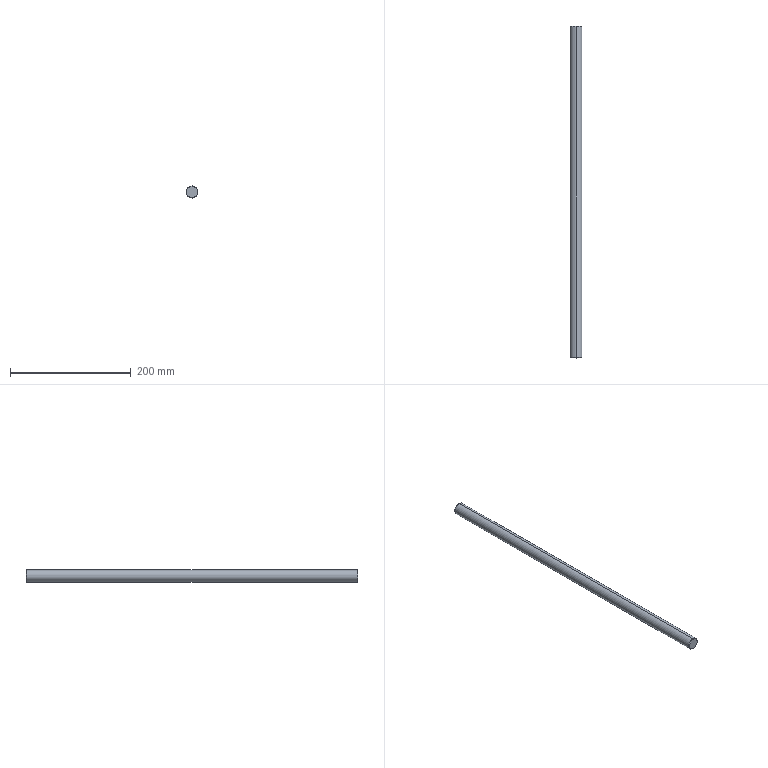Part | STEP file | BCC3 H16_11 | 1 solid | 8 faces | box 20 x 550 x 20 mm | volume 172727 mm3 | cone 4 | cylinder 2 | plane 2 | commonest cylinder face diameters 20 x2
STEP:
#1=CARTESIAN_POINT('',(0.,0.,0.));
#2=DIRECTION('',(0.,0.,1.));
#3=DIRECTION('',(1.,0.,0.));
#4=AXIS2_PLACEMENT_3D('',#1,#2,#3);
#5=CARTESIAN_POINT('',(0.,550.,9.));
#6=VERTEX_POINT('',#5);
#7=CARTESIAN_POINT('',(0.,550.,-9.));
#8=VERTEX_POINT('',#7);
#9=CARTESIAN_POINT('',(0.,550.,0.));
#10=DIRECTION('',(0.,1.,0.));
#11=DIRECTION('',(0.,0.,1.));
#12=AXIS2_PLACEMENT_3D('',#9,#10,#11);
#13=CIRCLE('',#12,9.);
#14=CARTESIAN_POINT('',(0.,550.,0.));
#15=DIRECTION('',(0.,-1.,0.));
#16=DIRECTION('',(0.,0.,-1.));
#17=AXIS2_PLACEMENT_3D('',#14,#15,#16);
#18=CONICAL_SURFACE('',#17,9.,0.7854);
#19=CARTESIAN_POINT('',(3.142,0.));
#20=DIRECTION('',(-1.,0.));
#21=VECTOR('',#20,1.);
#22=LINE('',#19,#21);
#23=(GEOMETRIC_REPRESENTATION_CONTEXT(2)PARAMETRIC_REPRESENTATION_CONTEXT()REPRESENTATION_CONTEXT('',''));
#24=DEFINITIONAL_REPRESENTATION('',(#22),#23);
#25=PCURVE('',#18,#24);
#26=CARTESIAN_POINT('',(0.,550.,0.));
#27=DIRECTION('',(0.,1.,0.));
#28=DIRECTION('',(0.,0.,1.));
#29=AXIS2_PLACEMENT_3D('',#26,#27,#28);
#30=PLANE('',#29);
#31=CARTESIAN_POINT('',(0.,0.));
#32=DIRECTION('',(1.,0.));
#33=AXIS2_PLACEMENT_2D('',#31,#32);
#34=CIRCLE('',#33,9.);
#35=(GEOMETRIC_REPRESENTATION_CONTEXT(2)PARAMETRIC_REPRESENTATION_CONTEXT()REPRESENTATION_CONTEXT('',''));
#36=DEFINITIONAL_REPRESENTATION('',(#34),#35);
#37=PCURVE('',#30,#36);
#38=SURFACE_CURVE('',#13,(#25,#37),.PCURVE_S1.);
#39=EDGE_CURVE('',#6,#8,#38,.T.);
#40=ORIENTED_EDGE('',*,*,#39,.F.);
#41=CARTESIAN_POINT('',(0.,549.,10.));
#42=VERTEX_POINT('',#41);
#43=CARTESIAN_POINT('',(0.,550.,9.));
#44=DIRECTION('',(0.,-0.7071,0.7071));
#45=VECTOR('',#44,1.);
#46=LINE('',#43,#45);
#47=CARTESIAN_POINT('',(3.142,0.));
#48=DIRECTION('',(0.,1.));
#49=VECTOR('',#48,1.);
#50=LINE('',#47,#49);
#51=(GEOMETRIC_REPRESENTATION_CONTEXT(2)PARAMETRIC_REPRESENTATION_CONTEXT()REPRESENTATION_CONTEXT('',''));
#52=DEFINITIONAL_REPRESENTATION('',(#50),#51);
#53=PCURVE('',#18,#52);
#54=CARTESIAN_POINT('',(0.,550.,0.));
#55=DIRECTION('',(0.,-1.,0.));
#56=DIRECTION('',(0.,0.,-1.));
#57=AXIS2_PLACEMENT_3D('',#54,#55,#56);
#58=CONICAL_SURFACE('',#57,9.,0.7854);
#59=CARTESIAN_POINT('',(3.142,0.));
#60=DIRECTION('',(0.,1.));
#61=VECTOR('',#60,1.);
#62=LINE('',#59,#61);
#63=(GEOMETRIC_REPRESENTATION_CONTEXT(2)PARAMETRIC_REPRESENTATION_CONTEXT()REPRESENTATION_CONTEXT('',''));
#64=DEFINITIONAL_REPRESENTATION('',(#62),#63);
#65=PCURVE('',#58,#64);
#66=SURFACE_CURVE('',#46,(#53,#65),.PCURVE_S1.);
#67=EDGE_CURVE('',#6,#42,#66,.T.);
#68=ORIENTED_EDGE('',*,*,#67,.T.);
#69=CARTESIAN_POINT('',(0.,549.,-10.));
#70=VERTEX_POINT('',#69);
#71=CARTESIAN_POINT('',(0.,549.,0.));
#72=DIRECTION('',(0.,-1.,0.));
#73=DIRECTION('',(0.,0.,1.));
#74=AXIS2_PLACEMENT_3D('',#71,#72,#73);
#75=CIRCLE('',#74,10.);
#76=CARTESIAN_POINT('',(-3.142,1.));
#77=DIRECTION('',(1.,0.));
#78=VECTOR('',#77,1.);
#79=LINE('',#76,#78);
#80=(GEOMETRIC_REPRESENTATION_CONTEXT(2)PARAMETRIC_REPRESENTATION_CONTEXT()REPRESENTATION_CONTEXT('',''));
#81=DEFINITIONAL_REPRESENTATION('',(#79),#80);
#82=PCURVE('',#18,#81);
#83=CARTESIAN_POINT('',(0.,550.,0.));
#84=DIRECTION('',(0.,-1.,0.));
#85=DIRECTION('',(0.,0.,-1.));
#86=AXIS2_PLACEMENT_3D('',#83,#84,#85);
#87=CYLINDRICAL_SURFACE('',#86,10.);
#88=CARTESIAN_POINT('',(-3.142,1.));
#89=DIRECTION('',(1.,0.));
#90=VECTOR('',#89,1.);
#91=LINE('',#88,#90);
#92=(GEOMETRIC_REPRESENTATION_CONTEXT(2)PARAMETRIC_REPRESENTATION_CONTEXT()REPRESENTATION_CONTEXT('',''));
#93=DEFINITIONAL_REPRESENTATION('',(#91),#92);
#94=PCURVE('',#87,#93);
#95=SURFACE_CURVE('',#75,(#82,#94),.PCURVE_S1.);
#96=EDGE_CURVE('',#70,#42,#95,.T.);
#97=ORIENTED_EDGE('',*,*,#96,.F.);
#98=CARTESIAN_POINT('',(0.,550.,-9.));
#99=DIRECTION('',(0.,-0.7071,-0.7071));
#100=VECTOR('',#99,1.);
#101=LINE('',#98,#100);
#102=CARTESIAN_POINT('',(0.,0.));
#103=DIRECTION('',(0.,1.));
#104=VECTOR('',#103,1.);
#105=LINE('',#102,#104);
#106=(GEOMETRIC_REPRESENTATION_CONTEXT(2)PARAMETRIC_REPRESENTATION_CONTEXT()REPRESENTATION_CONTEXT('',''));
#107=DEFINITIONAL_REPRESENTATION('',(#105),#106);
#108=PCURVE('',#18,#107);
#109=CARTESIAN_POINT('',(6.283,0.));
#110=DIRECTION('',(0.,1.));
#111=VECTOR('',#110,1.);
#112=LINE('',#109,#111);
#113=(GEOMETRIC_REPRESENTATION_CONTEXT(2)PARAMETRIC_REPRESENTATION_CONTEXT()REPRESENTATION_CONTEXT('',''));
#114=DEFINITIONAL_REPRESENTATION('',(#112),#113);
#115=PCURVE('',#58,#114);
#116=SURFACE_CURVE('',#101,(#108,#115),.PCURVE_S1.);
#117=EDGE_CURVE('',#8,#70,#116,.T.);
#118=ORIENTED_EDGE('',*,*,#117,.F.);
#119=EDGE_LOOP('',(#40,#68,#97,#118));
#120=FACE_BOUND('',#119,.T.);
#121=ADVANCED_FACE('',(#120),#18,.T.);
#122=CARTESIAN_POINT('',(0.,0.,-9.));
#123=VERTEX_POINT('',#122);
#124=CARTESIAN_POINT('',(0.,0.,9.));
#125=VERTEX_POINT('',#124);
#126=CARTESIAN_POINT('',(0.,0.,0.));
#127=DIRECTION('',(0.,-1.,0.));
#128=DIRECTION('',(0.,0.,1.));
#129=AXIS2_PLACEMENT_3D('',#126,#127,#128);
#130=CIRCLE('',#129,9.);
#131=CARTESIAN_POINT('',(0.,1.,0.));
#132=DIRECTION('',(0.,1.,0.));
#133=DIRECTION('',(0.,0.,1.));
#134=AXIS2_PLACEMENT_3D('',#131,#132,#133);
#135=CONICAL_SURFACE('',#134,10.,0.7854);
#136=CARTESIAN_POINT('',(6.283,-1.));
#137=DIRECTION('',(-1.,0.));
#138=VECTOR('',#137,1.);
#139=LINE('',#136,#138);
#140=(GEOMETRIC_REPRESENTATION_CONTEXT(2)PARAMETRIC_REPRESENTATION_CONTEXT()REPRESENTATION_CONTEXT('',''));
#141=DEFINITIONAL_REPRESENTATION('',(#139),#140);
#142=PCURVE('',#135,#141);
#143=CARTESIAN_POINT('',(0.,0.,0.));
#144=DIRECTION('',(0.,1.,0.));
#145=DIRECTION('',(0.,0.,1.));
#146=AXIS2_PLACEMENT_3D('',#143,#144,#145);
#147=PLANE('',#146);
#148=CARTESIAN_POINT('',(9.,0.));
#149=CARTESIAN_POINT('',(9.,-15.588));
#150=CARTESIAN_POINT('',(-4.5,-7.794));
#151=CARTESIAN_POINT('',(-18.,0.));
#152=CARTESIAN_POINT('',(-4.5,7.794));
#153=CARTESIAN_POINT('',(9.,15.588));
#154=CARTESIAN_POINT('',(9.,0.));
#155=(BOUNDED_CURVE()B_SPLINE_CURVE(2,(#148,#149,#150,#151,#152,#153,#154),.UNSPECIFIED.,.T.,.F.)B_SPLINE_CURVE_WITH_KNOTS((1,2,2,2,2,1),(-2.094,0.,2.094,4.189,6.283,8.378),.UNSPECIFIED.)CURVE()GEOMETRIC_REPRESENTATION_ITEM()RATIONAL_B_SPLINE_CURVE((1.,0.5,1.,0.5,1.,0.5,1.))REPRESENTATION_ITEM(''));
#156=(GEOMETRIC_REPRESENTATION_CONTEXT(2)PARAMETRIC_REPRESENTATION_CONTEXT()REPRESENTATION_CONTEXT('',''));
#157=DEFINITIONAL_REPRESENTATION('',(#155),#156);
#158=PCURVE('',#147,#157);
#159=SURFACE_CURVE('',#130,(#142,#158),.PCURVE_S1.);
#160=EDGE_CURVE('',#123,#125,#159,.T.);
#161=ORIENTED_EDGE('',*,*,#160,.F.);
#162=CARTESIAN_POINT('',(0.,1.,-10.));
#163=VERTEX_POINT('',#162);
#164=CARTESIAN_POINT('',(0.,1.,-10.));
#165=DIRECTION('',(0.,0.7071,-0.7071));
#166=VECTOR('',#165,1.);
#167=LINE('',#164,#166);
#168=CARTESIAN_POINT('',(3.142,0.));
#169=DIRECTION('',(0.,1.));
#170=VECTOR('',#169,1.);
#171=LINE('',#168,#170);
#172=(GEOMETRIC_REPRESENTATION_CONTEXT(2)PARAMETRIC_REPRESENTATION_CONTEXT()REPRESENTATION_CONTEXT('',''));
#173=DEFINITIONAL_REPRESENTATION('',(#171),#172);
#174=PCURVE('',#135,#173);
#175=CARTESIAN_POINT('',(0.,1.,0.));
#176=DIRECTION('',(0.,1.,0.));
#177=DIRECTION('',(0.,0.,1.));
#178=AXIS2_PLACEMENT_3D('',#175,#176,#177);
#179=CONICAL_SURFACE('',#178,10.,0.7854);
#180=CARTESIAN_POINT('',(3.142,0.));
#181=DIRECTION('',(0.,1.));
#182=VECTOR('',#181,1.);
#183=LINE('',#180,#182);
#184=(GEOMETRIC_REPRESENTATION_CONTEXT(2)PARAMETRIC_REPRESENTATION_CONTEXT()REPRESENTATION_CONTEXT('',''));
#185=DEFINITIONAL_REPRESENTATION('',(#183),#184);
#186=PCURVE('',#179,#185);
#187=SURFACE_CURVE('',#167,(#174,#186),.PCURVE_S1.);
#188=EDGE_CURVE('',#123,#163,#187,.T.);
#189=ORIENTED_EDGE('',*,*,#188,.T.);
#190=CARTESIAN_POINT('',(0.,1.,10.));
#191=VERTEX_POINT('',#190);
#192=CARTESIAN_POINT('',(0.,1.,0.));
#193=DIRECTION('',(0.,1.,0.));
#194=DIRECTION('',(0.,0.,1.));
#195=AXIS2_PLACEMENT_3D('',#192,#193,#194);
#196=CIRCLE('',#195,10.);
#197=CARTESIAN_POINT('',(0.,0.));
#198=DIRECTION('',(1.,0.));
#199=VECTOR('',#198,1.);
#200=LINE('',#197,#199);
#201=(GEOMETRIC_REPRESENTATION_CONTEXT(2)PARAMETRIC_REPRESENTATION_CONTEXT()REPRESENTATION_CONTEXT('',''));
#202=DEFINITIONAL_REPRESENTATION('',(#200),#201);
#203=PCURVE('',#135,#202);
#204=CARTESIAN_POINT('',(3.142,549.));
#205=DIRECTION('',(-1.,0.));
#206=VECTOR('',#205,1.);
#207=LINE('',#204,#206);
#208=(GEOMETRIC_REPRESENTATION_CONTEXT(2)PARAMETRIC_REPRESENTATION_CONTEXT()REPRESENTATION_CONTEXT('',''));
#209=DEFINITIONAL_REPRESENTATION('',(#207),#208);
#210=PCURVE('',#87,#209);
#211=SURFACE_CURVE('',#196,(#203,#210),.PCURVE_S1.);
#212=EDGE_CURVE('',#191,#163,#211,.T.);
#213=ORIENTED_EDGE('',*,*,#212,.F.);
#214=CARTESIAN_POINT('',(0.,1.,10.));
#215=DIRECTION('',(0.,0.7071,0.7071));
#216=VECTOR('',#215,1.);
#217=LINE('',#214,#216);
#218=CARTESIAN_POINT('',(0.,0.));
#219=DIRECTION('',(0.,1.));
#220=VECTOR('',#219,1.);
#221=LINE('',#218,#220);
#222=(GEOMETRIC_REPRESENTATION_CONTEXT(2)PARAMETRIC_REPRESENTATION_CONTEXT()REPRESENTATION_CONTEXT('',''));
#223=DEFINITIONAL_REPRESENTATION('',(#221),#222);
#224=PCURVE('',#135,#223);
#225=CARTESIAN_POINT('',(6.283,0.));
#226=DIRECTION('',(0.,1.));
#227=VECTOR('',#226,1.);
#228=LINE('',#225,#227);
#229=(GEOMETRIC_REPRESENTATION_CONTEXT(2)PARAMETRIC_REPRESENTATION_CONTEXT()REPRESENTATION_CONTEXT('',''));
#230=DEFINITIONAL_REPRESENTATION('',(#228),#229);
#231=PCURVE('',#179,#230);
#232=SURFACE_CURVE('',#217,(#224,#231),.PCURVE_S1.);
#233=EDGE_CURVE('',#125,#191,#232,.T.);
#234=ORIENTED_EDGE('',*,*,#233,.F.);
#235=EDGE_LOOP('',(#161,#189,#213,#234));
#236=FACE_BOUND('',#235,.T.);
#237=ADVANCED_FACE('',(#236),#135,.T.);
#238=ORIENTED_EDGE('',*,*,#96,.T.);
#239=CARTESIAN_POINT('',(0.,550.,10.));
#240=DIRECTION('',(0.,-1.,0.));
#241=VECTOR('',#240,1.);
#242=LINE('',#239,#241);
#243=CARTESIAN_POINT('',(3.142,0.));
#244=DIRECTION('',(0.,1.));
#245=VECTOR('',#244,1.);
#246=LINE('',#243,#245);
#247=(GEOMETRIC_REPRESENTATION_CONTEXT(2)PARAMETRIC_REPRESENTATION_CONTEXT()REPRESENTATION_CONTEXT('',''));
#248=DEFINITIONAL_REPRESENTATION('',(#246),#247);
#249=PCURVE('',#87,#248);
#250=CARTESIAN_POINT('',(0.,550.,0.));
#251=DIRECTION('',(0.,-1.,0.));
#252=DIRECTION('',(0.,0.,-1.));
#253=AXIS2_PLACEMENT_3D('',#250,#251,#252);
#254=CYLINDRICAL_SURFACE('',#253,10.);
#255=CARTESIAN_POINT('',(3.142,0.));
#256=DIRECTION('',(0.,1.));
#257=VECTOR('',#256,1.);
#258=LINE('',#255,#257);
#259=(GEOMETRIC_REPRESENTATION_CONTEXT(2)PARAMETRIC_REPRESENTATION_CONTEXT()REPRESENTATION_CONTEXT('',''));
#260=DEFINITIONAL_REPRESENTATION('',(#258),#259);
#261=PCURVE('',#254,#260);
#262=SURFACE_CURVE('',#242,(#249,#261),.PCURVE_S1.);
#263=EDGE_CURVE('',#42,#191,#262,.T.);
#264=ORIENTED_EDGE('',*,*,#263,.T.);
#265=ORIENTED_EDGE('',*,*,#212,.T.);
#266=CARTESIAN_POINT('',(0.,550.,-10.));
#267=DIRECTION('',(0.,-1.,0.));
#268=VECTOR('',#267,1.);
#269=LINE('',#266,#268);
#270=CARTESIAN_POINT('',(0.,0.));
#271=DIRECTION('',(0.,1.));
#272=VECTOR('',#271,1.);
#273=LINE('',#270,#272);
#274=(GEOMETRIC_REPRESENTATION_CONTEXT(2)PARAMETRIC_REPRESENTATION_CONTEXT()REPRESENTATION_CONTEXT('',''));
#275=DEFINITIONAL_REPRESENTATION('',(#273),#274);
#276=PCURVE('',#87,#275);
#277=CARTESIAN_POINT('',(6.283,0.));
#278=DIRECTION('',(0.,1.));
#279=VECTOR('',#278,1.);
#280=LINE('',#277,#279);
#281=(GEOMETRIC_REPRESENTATION_CONTEXT(2)PARAMETRIC_REPRESENTATION_CONTEXT()REPRESENTATION_CONTEXT('',''));
#282=DEFINITIONAL_REPRESENTATION('',(#280),#281);
#283=PCURVE('',#254,#282);
#284=SURFACE_CURVE('',#269,(#276,#283),.PCURVE_S1.);
#285=EDGE_CURVE('',#70,#163,#284,.T.);
#286=ORIENTED_EDGE('',*,*,#285,.F.);
#287=EDGE_LOOP('',(#238,#264,#265,#286));
#288=FACE_BOUND('',#287,.T.);
#289=ADVANCED_FACE('',(#288),#87,.T.);
#290=ORIENTED_EDGE('',*,*,#263,.F.);
#291=CARTESIAN_POINT('',(0.,549.,0.));
#292=DIRECTION('',(0.,-1.,0.));
#293=DIRECTION('',(0.,0.,1.));
#294=AXIS2_PLACEMENT_3D('',#291,#292,#293);
#295=CIRCLE('',#294,10.);
#296=CARTESIAN_POINT('',(3.142,1.));
#297=DIRECTION('',(1.,0.));
#298=VECTOR('',#297,1.);
#299=LINE('',#296,#298);
#300=(GEOMETRIC_REPRESENTATION_CONTEXT(2)PARAMETRIC_REPRESENTATION_CONTEXT()REPRESENTATION_CONTEXT('',''));
#301=DEFINITIONAL_REPRESENTATION('',(#299),#300);
#302=PCURVE('',#254,#301);
#303=CARTESIAN_POINT('',(3.142,1.));
#304=DIRECTION('',(1.,0.));
#305=VECTOR('',#304,1.);
#306=LINE('',#303,#305);
#307=(GEOMETRIC_REPRESENTATION_CONTEXT(2)PARAMETRIC_REPRESENTATION_CONTEXT()REPRESENTATION_CONTEXT('',''));
#308=DEFINITIONAL_REPRESENTATION('',(#306),#307);
#309=PCURVE('',#58,#308);
#310=SURFACE_CURVE('',#295,(#302,#309),.PCURVE_S1.);
#311=EDGE_CURVE('',#42,#70,#310,.T.);
#312=ORIENTED_EDGE('',*,*,#311,.T.);
#313=ORIENTED_EDGE('',*,*,#285,.T.);
#314=CARTESIAN_POINT('',(0.,1.,0.));
#315=DIRECTION('',(0.,1.,0.));
#316=DIRECTION('',(0.,0.,1.));
#317=AXIS2_PLACEMENT_3D('',#314,#315,#316);
#318=CIRCLE('',#317,10.);
#319=CARTESIAN_POINT('',(9.425,549.));
#320=DIRECTION('',(-1.,0.));
#321=VECTOR('',#320,1.);
#322=LINE('',#319,#321);
#323=(GEOMETRIC_REPRESENTATION_CONTEXT(2)PARAMETRIC_REPRESENTATION_CONTEXT()REPRESENTATION_CONTEXT('',''));
#324=DEFINITIONAL_REPRESENTATION('',(#322),#323);
#325=PCURVE('',#254,#324);
#326=CARTESIAN_POINT('',(0.,0.));
#327=DIRECTION('',(1.,0.));
#328=VECTOR('',#327,1.);
#329=LINE('',#326,#328);
#330=(GEOMETRIC_REPRESENTATION_CONTEXT(2)PARAMETRIC_REPRESENTATION_CONTEXT()REPRESENTATION_CONTEXT('',''));
#331=DEFINITIONAL_REPRESENTATION('',(#329),#330);
#332=PCURVE('',#179,#331);
#333=SURFACE_CURVE('',#318,(#325,#332),.PCURVE_S1.);
#334=EDGE_CURVE('',#163,#191,#333,.T.);
#335=ORIENTED_EDGE('',*,*,#334,.T.);
#336=EDGE_LOOP('',(#290,#312,#313,#335));
#337=FACE_BOUND('',#336,.T.);
#338=ADVANCED_FACE('',(#337),#254,.T.);
#339=CARTESIAN_POINT('',(0.,550.,0.));
#340=DIRECTION('',(0.,1.,0.));
#341=DIRECTION('',(0.,0.,1.));
#342=AXIS2_PLACEMENT_3D('',#339,#340,#341);
#343=CIRCLE('',#342,9.);
#344=CARTESIAN_POINT('',(0.,0.));
#345=DIRECTION('',(1.,0.));
#346=AXIS2_PLACEMENT_2D('',#344,#345);
#347=CIRCLE('',#346,9.);
#348=(GEOMETRIC_REPRESENTATION_CONTEXT(2)PARAMETRIC_REPRESENTATION_CONTEXT()REPRESENTATION_CONTEXT('',''));
#349=DEFINITIONAL_REPRESENTATION('',(#347),#348);
#350=PCURVE('',#30,#349);
#351=CARTESIAN_POINT('',(9.425,0.));
#352=DIRECTION('',(-1.,0.));
#353=VECTOR('',#352,1.);
#354=LINE('',#351,#353);
#355=(GEOMETRIC_REPRESENTATION_CONTEXT(2)PARAMETRIC_REPRESENTATION_CONTEXT()REPRESENTATION_CONTEXT('',''));
#356=DEFINITIONAL_REPRESENTATION('',(#354),#355);
#357=PCURVE('',#58,#356);
#358=SURFACE_CURVE('',#343,(#350,#357),.PCURVE_S1.);
#359=EDGE_CURVE('',#8,#6,#358,.T.);
#360=ORIENTED_EDGE('',*,*,#359,.T.);
#361=ORIENTED_EDGE('',*,*,#39,.T.);
#362=EDGE_LOOP('',(#360,#361));
#363=FACE_BOUND('',#362,.T.);
#364=ADVANCED_FACE('',(#363),#30,.T.);
#365=CARTESIAN_POINT('',(0.,0.,0.));
#366=DIRECTION('',(0.,-1.,0.));
#367=DIRECTION('',(0.,0.,1.));
#368=AXIS2_PLACEMENT_3D('',#365,#366,#367);
#369=CIRCLE('',#368,9.);
#370=CARTESIAN_POINT('',(9.,0.));
#371=CARTESIAN_POINT('',(9.,-15.588));
#372=CARTESIAN_POINT('',(-4.5,-7.794));
#373=CARTESIAN_POINT('',(-18.,0.));
#374=CARTESIAN_POINT('',(-4.5,7.794));
#375=CARTESIAN_POINT('',(9.,15.588));
#376=CARTESIAN_POINT('',(9.,0.));
#377=(BOUNDED_CURVE()B_SPLINE_CURVE(2,(#370,#371,#372,#373,#374,#375,#376),.UNSPECIFIED.,.T.,.F.)B_SPLINE_CURVE_WITH_KNOTS((1,2,2,2,2,1),(-2.094,0.,2.094,4.189,6.283,8.378),.UNSPECIFIED.)CURVE()GEOMETRIC_REPRESENTATION_ITEM()RATIONAL_B_SPLINE_CURVE((1.,0.5,1.,0.5,1.,0.5,1.))REPRESENTATION_ITEM(''));
#378=(GEOMETRIC_REPRESENTATION_CONTEXT(2)PARAMETRIC_REPRESENTATION_CONTEXT()REPRESENTATION_CONTEXT('',''));
#379=DEFINITIONAL_REPRESENTATION('',(#377),#378);
#380=PCURVE('',#147,#379);
#381=CARTESIAN_POINT('',(6.283,-1.));
#382=DIRECTION('',(-1.,0.));
#383=VECTOR('',#382,1.);
#384=LINE('',#381,#383);
#385=(GEOMETRIC_REPRESENTATION_CONTEXT(2)PARAMETRIC_REPRESENTATION_CONTEXT()REPRESENTATION_CONTEXT('',''));
#386=DEFINITIONAL_REPRESENTATION('',(#384),#385);
#387=PCURVE('',#179,#386);
#388=SURFACE_CURVE('',#369,(#380,#387),.PCURVE_S1.);
#389=EDGE_CURVE('',#125,#123,#388,.T.);
#390=ORIENTED_EDGE('',*,*,#389,.T.);
#391=ORIENTED_EDGE('',*,*,#160,.T.);
#392=EDGE_LOOP('',(#390,#391));
#393=FACE_BOUND('',#392,.T.);
#394=ADVANCED_FACE('',(#393),#147,.F.);
#395=ORIENTED_EDGE('',*,*,#188,.F.);
#396=ORIENTED_EDGE('',*,*,#389,.F.);
#397=ORIENTED_EDGE('',*,*,#233,.T.);
#398=ORIENTED_EDGE('',*,*,#334,.F.);
#399=EDGE_LOOP('',(#395,#396,#397,#398));
#400=FACE_BOUND('',#399,.T.);
#401=ADVANCED_FACE('',(#400),#179,.T.);
#402=ORIENTED_EDGE('',*,*,#67,.F.);
#403=ORIENTED_EDGE('',*,*,#359,.F.);
#404=ORIENTED_EDGE('',*,*,#117,.T.);
#405=ORIENTED_EDGE('',*,*,#311,.F.);
#406=EDGE_LOOP('',(#402,#403,#404,#405));
#407=FACE_BOUND('',#406,.T.);
#408=ADVANCED_FACE('',(#407),#58,.T.);
#409=CLOSED_SHELL('',(#121,#237,#289,#338,#364,#394,#401,#408));
#410=MANIFOLD_SOLID_BREP('',#409);
#411=(LENGTH_UNIT()NAMED_UNIT(*)SI_UNIT(.MILLI.,.METRE.));
#412=UNCERTAINTY_MEASURE_WITH_UNIT(LENGTH_MEASURE(0.0000001),#411,'','');
#413=(NAMED_UNIT(*)PLANE_ANGLE_UNIT()SI_UNIT($,.RADIAN.));
#414=(NAMED_UNIT(*)SI_UNIT($,.STERADIAN.)SOLID_ANGLE_UNIT());
#415=(GEOMETRIC_REPRESENTATION_CONTEXT(3)GLOBAL_UNCERTAINTY_ASSIGNED_CONTEXT((#412))GLOBAL_UNIT_ASSIGNED_CONTEXT((#411,#413,#414))REPRESENTATION_CONTEXT('',''));
#416=ADVANCED_BREP_SHAPE_REPRESENTATION('',(#4,#410),#415);